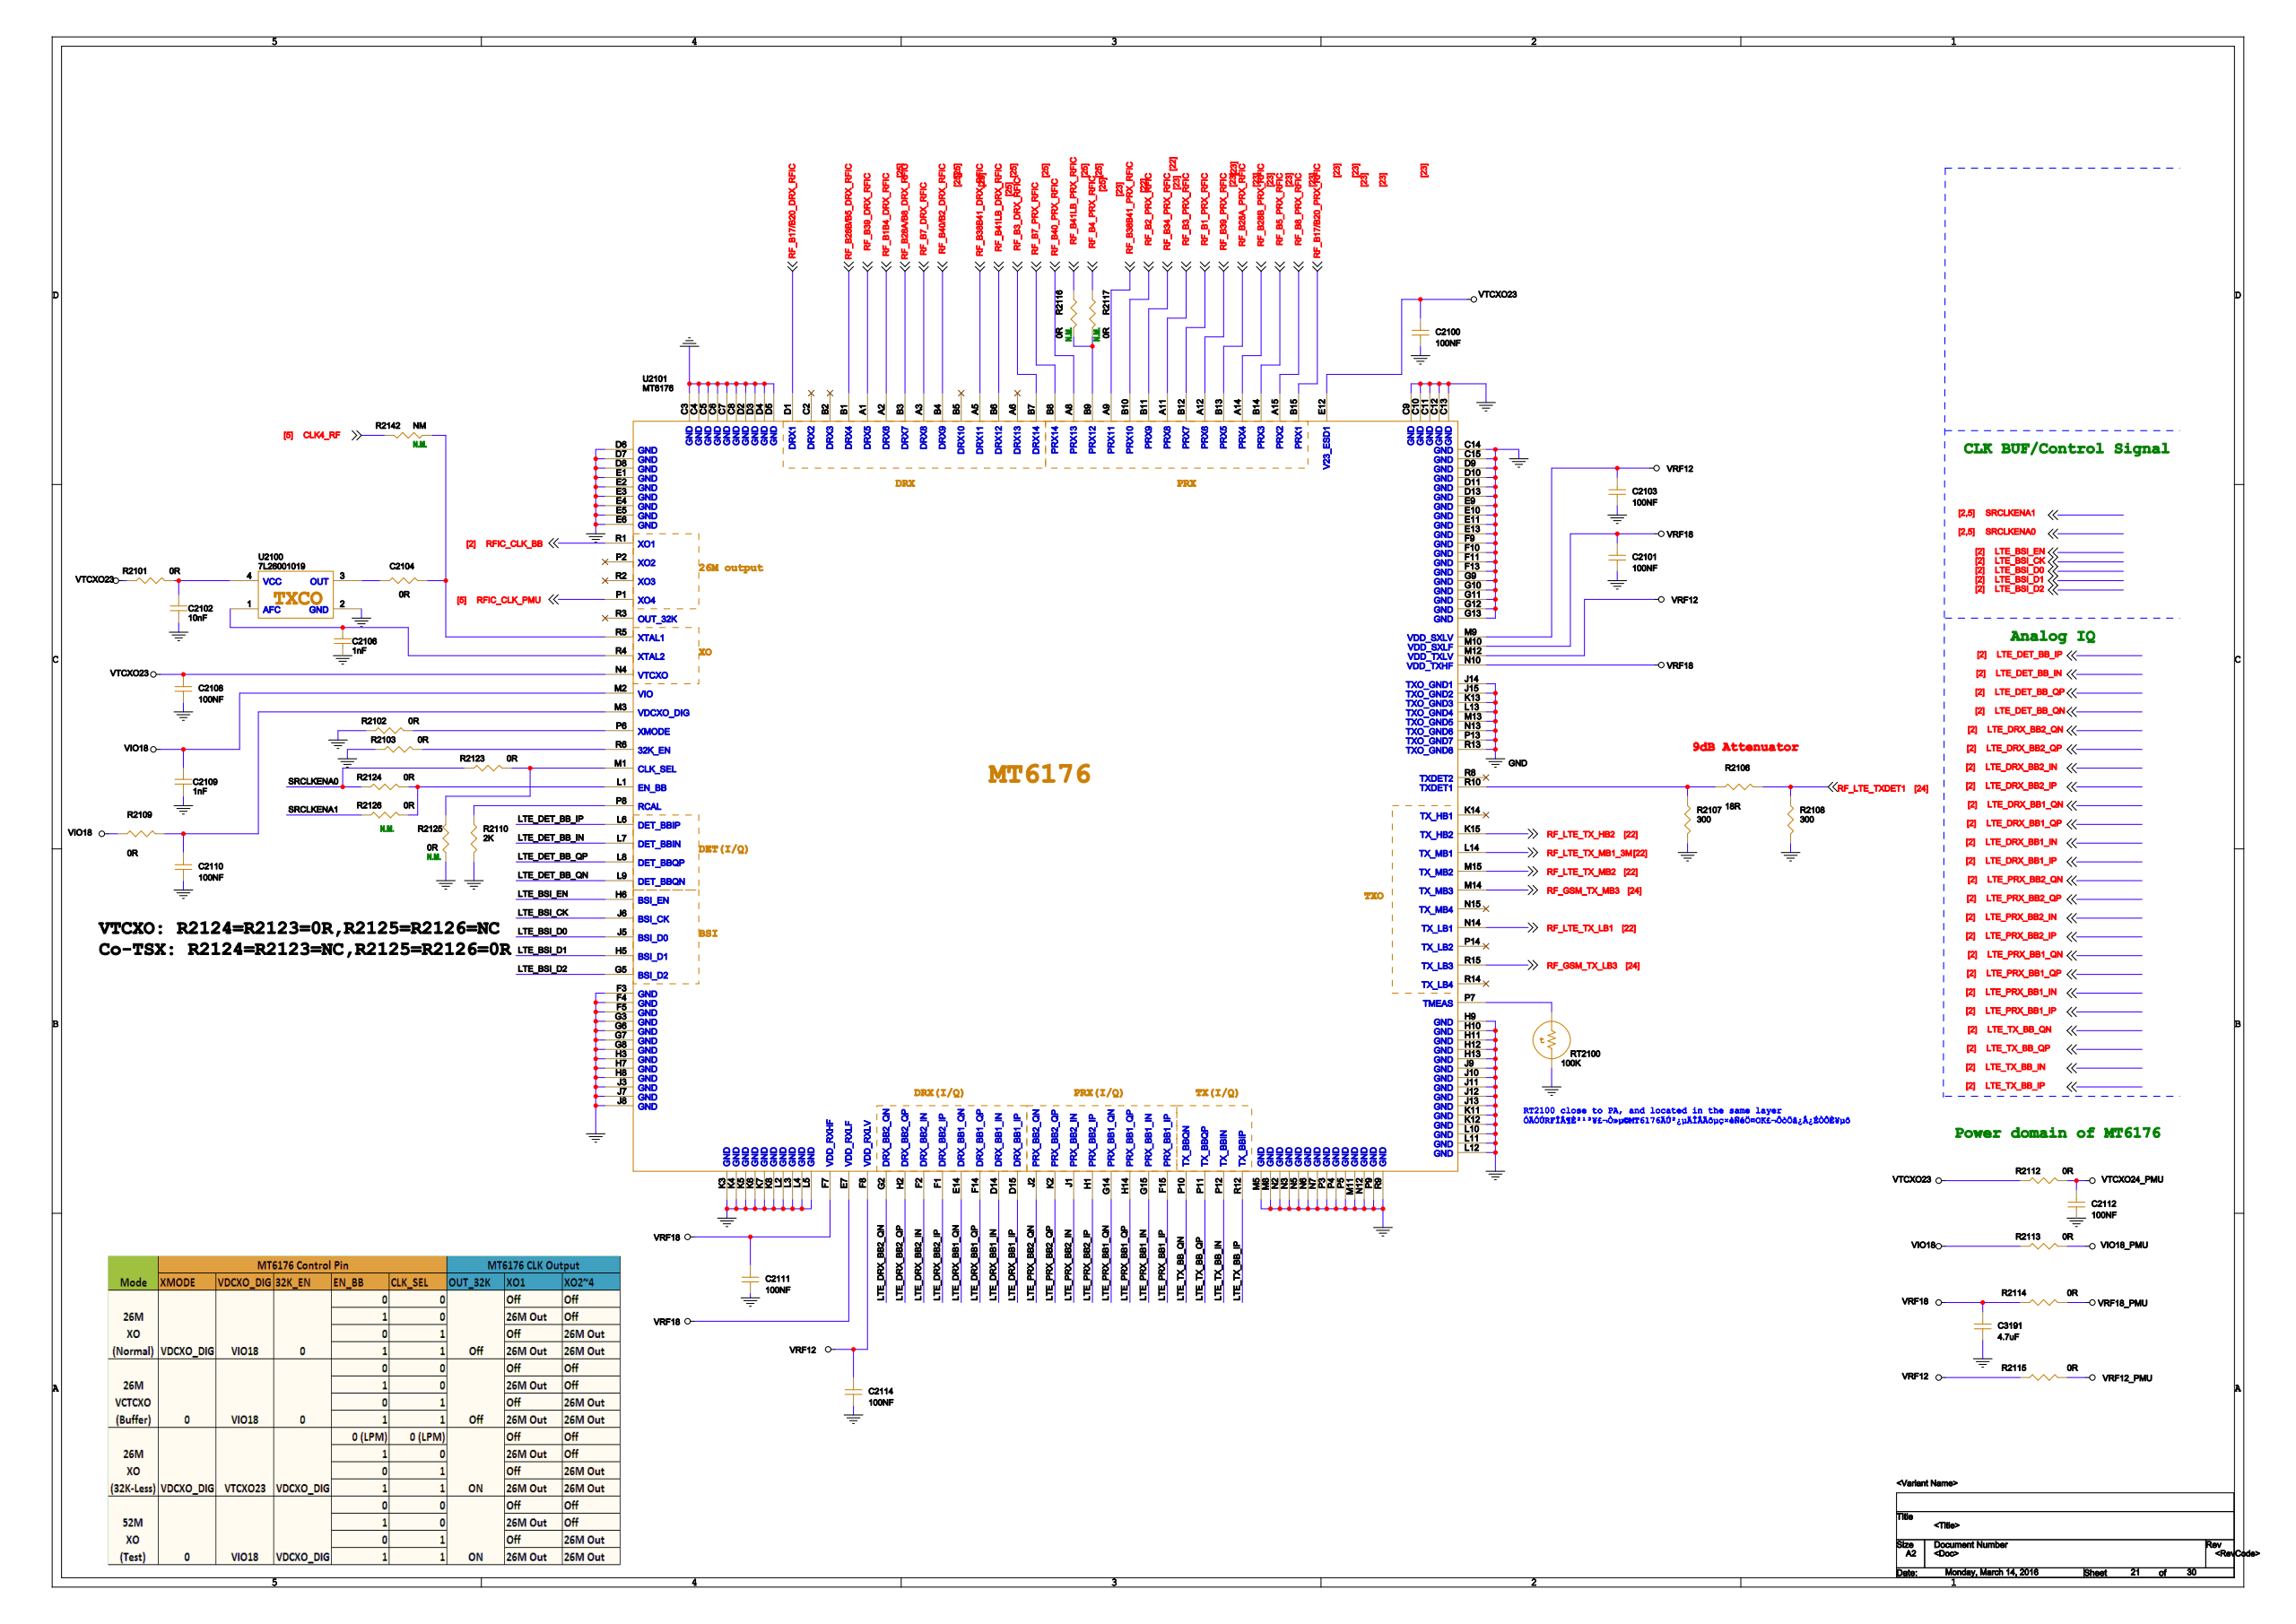Circuit board | Cadence Allegro | 1088 parts | 793 nets | one sheet of the schematic
Parts on this sheet (reference | value | footprint):
C2100 | 100NF | C0201
C2101 | 100NF | C0201
C2102 | 10nF | C0201
C2103 | 100NF | C0201
C2104 | 0R | R0201
C2106 | 1nF | C0201
C2108 | 100NF | C0201
C2109 | 1nF | C0201
C2110 | 100NF | C0201
C2111 | 100NF | C0201
C2112 | 100NF | C0201
C2114 | 100NF | C0201
C3191 | 4.7uF | 0402-BIG
R2101 | 0R | R0201
R2102 | 0R | R0201
R2103 | 0R | R0201
R2106 | 18R | R0201
R2107 | 300 | R0201
R2108 | 300 | R0201
R2109 | 0R | R0201
R2110 | 2K | R0201
R2112 | 0R | R0201
R2113 | 0R | R0201
R2114 | 0R | R0402
R2115 | 0R | R0402
R2116
R2117
R2123 | 0R | R0201
R2124 | 0R | R0201
R2125
R2126
R2142
RT2100 | 100k | R0201
U2100 | 7L26001019 | Y4_7L26002009
U2101 | MT6176 | VFBGA196_6P2X6P2X1_0P4
Nets of these parts (net: part-pin ...):
GND: C2100-1 C2101-1 C2102-2 C2103-1 C2106-2 C2108-1 C2109-2 C2110-1 C2111-1 C2112-1 C2114-1 C3191-1 R2102-1 R2103-1 R2107-2 R2108-2 R2110-2 R2125-1 RT2100-2 U2100-2 U2101-C3 U2101-C4 U2101-C5 U2101-C6 U2101-C7 U2101-C8 U2101-C9 U2101-C10 U2101-C11 U2101-C12 U2101-C14 U2101-C15 U2101-D2 U2101-D3 U2101-D4 U2101-D5 U2101-D6 U2101-D7 U2101-D8 U2101-D9 U2101-D10 U2101-D11 U2101-D13 U2101-E1 U2101-E2 U2101-E3 U2101-E4 U2101-E5 U2101-E6 U2101-E9 U2101-E10 U2101-E11 U2101-E13 U2101-F3 U2101-F4 U2101-F5 U2101-F9 U2101-F10 U2101-F11 U2101-F13 U2101-G3 U2101-G6 U2101-G7 U2101-G8 U2101-G9 U2101-G10 U2101-G11 U2101-G12 U2101-G13 U2101-H3 U2101-H7 U2101-H8 U2101-H9 U2101-H10 U2101-H11 U2101-H12 U2101-H13 U2101-J3 U2101-J7 U2101-J8 U2101-J9 U2101-J10 U2101-J11 U2101-J12 U2101-J13 U2101-J14 U2101-J15 U2101-K3 U2101-K4 U2101-K5 U2101-K6 U2101-K7 U2101-K8 U2101-K11 U2101-K12 U2101-K13 U2101-L2 U2101-L3 U2101-L4 U2101-L5 U2101-L10 U2101-L11 U2101-L12 U2101-L13 U2101-M5 U2101-M8 U2101-M11 U2101-M13 U2101-N2 U2101-N3 U2101-N5 U2101-N6 U2101-N7 U2101-N12 U2101-N13 U2101-P3 U2101-P4 U2101-P5 U2101-P9 U2101-P13 U2101-R9 U2101-R13
N31493056: C2106-1 U2100-1 U2101-R4
N31494804: C2104-1 U2100-3
N31491381: C2102-1 R2101-2 U2100-4
SRCLKENA0: R2123-1 R2124-1
SRCLKENA1: R2126-1
LTE_DET_BB_IN: U2101-L7
LTE_DET_BB_IP: U2101-L6
LTE_DET_BB_QN: U2101-L9
LTE_DET_BB_QP: U2101-L8
LTE_DRX_BB1_IN: U2101-D14
LTE_DRX_BB1_IP: U2101-D15
LTE_DRX_BB1_QN: U2101-E14
LTE_DRX_BB1_QP: U2101-F14
LTE_DRX_BB2_IN: U2101-F2
LTE_DRX_BB2_IP: U2101-F1
LTE_DRX_BB2_QN: U2101-G2
LTE_DRX_BB2_QP: U2101-H2
LTE_PRX_BB1_IN: U2101-G15
LTE_PRX_BB1_IP: U2101-F15
LTE_PRX_BB1_QN: U2101-G14
LTE_PRX_BB1_QP: U2101-H14
LTE_PRX_BB2_IN: U2101-J1
LTE_PRX_BB2_IP: U2101-H1
LTE_PRX_BB2_QN: U2101-J2
LTE_PRX_BB2_QP: U2101-K2
LTE_BSI_CK: U2101-J6
LTE_BSI_D0: U2101-J5
LTE_BSI_D1: U2101-H5
LTE_BSI_D2: U2101-G5
LTE_BSI_EN: U2101-H6
LTE_TX_BB_IN: U2101-P12
LTE_TX_BB_IP: U2101-R12
LTE_TX_BB_QN: U2101-P10
LTE_TX_BB_QP: U2101-P11
VIO18_PMU: R2113-2
RF_LTE_TXDET1: R2106-2 R2108-1
N18204384: R2110-1 U2101-P8
N18204380: RT2100-1 U2101-P7
VTCXO24_PMU: C2112-2 R2112-2
VRF18: C2101-2 C2111-2 C3191-2 R2114-1 U2101-E7 U2101-F7 U2101-M10 U2101-N10
VRF18_PMU: R2114-2
VRF12_PMU: R2115-2
VTCXO23: C2100-2 C2108-2 R2101-1 R2112-1 U2101-E12 U2101-N4
VRF12: C2103-2 C2114-2 R2115-1 U2101-F8 U2101-M9 U2101-M12
N18204524: C2110-2 R2109-2 U2101-M3
RF_B2_PRX_RFIC: U2101-B10
RF_LTE_TX_MB2: U2101-M15
RF_LTE_TX_LB1: U2101-N14
RF_B5_PRX_RFIC: U2101-B14
RF_GSM_TX_LB3: U2101-R15
VIO18: C2109-1 R2109-1 R2113-1 U2101-M2
CLK4_RF: R2142-2
RF_LTE_TX_HB2: U2101-K15
RF_B28B_PRX_RFIC: U2101-A14
RF_B17/B20_PRX_RFIC: U2101-B15
RF_B38B41_PRX_RFIC: U2101-A9
RF_B8_PRX_RFIC: U2101-A15
RF_B39_PRX_RFIC: U2101-A12
RF_B4_PRX_RFIC: R2117-1
RF_B34_PRX_RFIC: U2101-B11
RF_B28A_PRX_RFIC: U2101-B13
RF_GSM_TX_MB3: U2101-M14
N18204301: C2104-2 R2142-1 U2101-R5
N18204149: R2106-1 R2107-1 U2101-R10
RFIC_CLK_PMU: U2101-P1
N18204750: R2103-2 U2101-R6
N33895670: R2123-2 R2125-2 U2101-M1
RF_B17/B20_DRX_RFIC: U2101-D1
RF_B38B41_DRX_RFIC: U2101-A5
RF_B41LB_DRX_RFIC: U2101-B6
RF_B3_DRX_RFIC: U2101-B7
RF_B28B/B5_DRX_RFIC: U2101-B1
RF_B39_DRX_RFIC: U2101-A1
RF_B1B4_DRX_RFIC: U2101-A2
RF_B28A/B8_DRX_RFIC: U2101-B3
RF_B7_DRX_RFIC: U2101-A3
RF_B40/B2_DRX_RFIC: U2101-B4
N18381162: R2124-2 R2126-2 U2101-L1
N31575151: R2116-2 R2117-2 U2101-B9
RF_B40_PRX_RFIC: U2101-A8
RF_B7_PRX_RFIC: U2101-B8
RF_B1_PRX_RFIC: U2101-B12
RF_B3_PRX_RFIC: U2101-A11
N18204341: R2102-2 U2101-P6
RFIC_CLK_BB: U2101-R1
RF_B41LB_PRX_RFIC: R2116-1